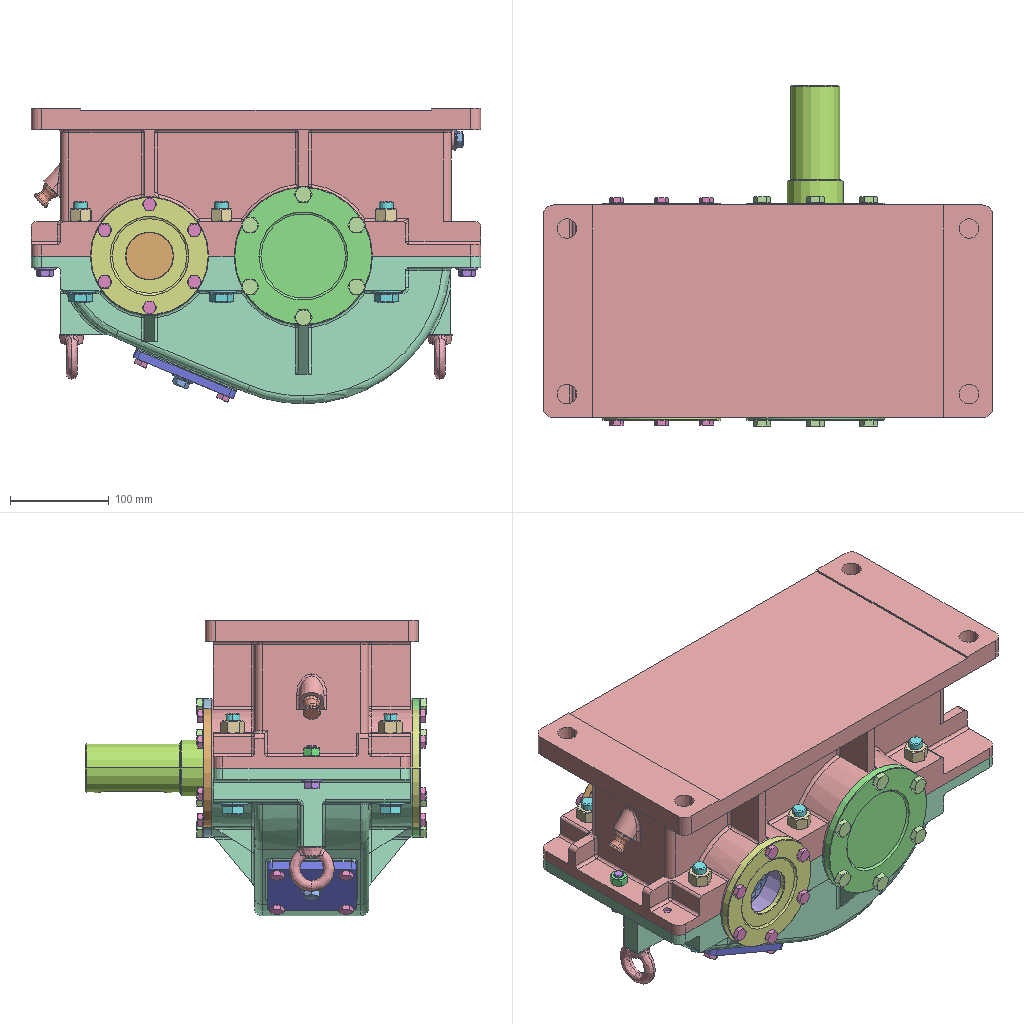Assembly | SolidWorks | 26 different items | 28 placed | box 456 x 346 x 300 mm
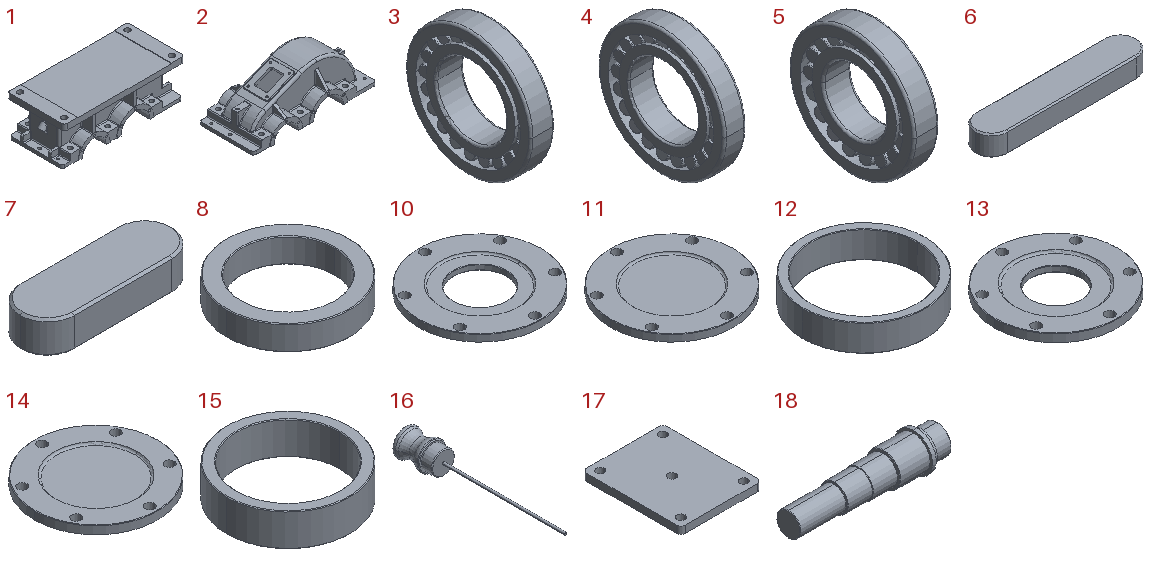Parts list (item | name | quantity | size | volume | features):
1 | - | x1 | 456 x 216 x 150 mm | 3465010 mm3 | features Fillet 25, ICE 15, 3DProfileFeature 4, HoleWzd 4, Chamfer 1, Extrusion 1, MirrorPattern 1, Sweep 1
2 | - | x1 | 456 x 204 x 150 mm | 1972353 mm3 | features Fillet 21, ICE 16, 3DProfileFeature 4, HoleWzd 4, Extrusion 1, MirrorPattern 1
3 | - | x1 | 21.75 x 90 x 90 mm | 63957 mm3 | features Revolution 3, CirPattern 1
4 | - | x1 | 23.75 x 110 x 110 mm | 105381 mm3 | features Revolution 3, CirPattern 1
5 | - | x1 | 19.75 x 80 x 80 mm | 50008 mm3 | features Revolution 3, CirPattern 1
6 | - | x1 | 70 x 14 x 9 mm | 8386 mm3 | features Boss 2, Chamfer 1, Extrusion 1
7 | - | x1 | 56 x 20 x 12 mm | 12325 mm3 | features Boss 2, Chamfer 1, Extrusion 1
8 | - | x1 | 80 x 80 x 16 mm | 35076 mm3 | features Chamfer 1, Extrusion 1
9 | - | x1 | - | - | features ICE 4, Boss 3, CirPattern 3, Cut 2, Fillet 2, Helix 2, SweepCut 2, Chamfer 1, Revolution 1
10 | - | x1 | 140 x 140 x 13 mm | 97648 mm3 | features ICE 3, Chamfer 2, Extrusion 1, Fillet 1
11 | - | x1 | 140 x 140 x 13 mm | 114660 mm3 | features ICE 2, Chamfer 1, Extrusion 1, Fillet 1
12 | - | x2 | 110 x 110 x 24 mm | 57801 mm3 | features Chamfer 1, Extrusion 1
13 | - | x1 | 120 x 120 x 13 mm | 73283 mm3 | features ICE 3, Chamfer 2, Extrusion 1, Fillet 1
14 | - | x1 | 120 x 120 x 13 mm | 84178 mm3 | features ICE 2, Chamfer 1, Extrusion 1, Fillet 1
15 | - | x2 | 90 x 90 x 24 mm | 46523 mm3 | features Chamfer 1, Extrusion 1
16 | - | x1 | 18 x 105 x 18 mm | 4726 mm3 | features Chamfer 2, Fillet 1, Revolution 1
17 | - | x1 | 90 x 110 x 8 mm | 76484 mm3 | features 3DProfileFeature 1, Extrusion 1, HoleWzd 1
18 | - | x1 | 312 x 80 x 80 mm | 861601 mm3 | features Chamfer 4, Fillet 2, ICE 2, Revolution 1
19 | eyebolts gb | x1 | - | - | -
20 | hex flange bolts-heavy grade b gb | x1 | - | - | -
21 | hex nuts, style 1-grades ab gb | x1 | - | - | -
22 | hexagon head bolts-full thread gb | x1 | - | - | -
23 | parallel pins hardening steel gb | x1 | - | - | -
24 | plain parallel keys | x1 | - | - | -
25 | tapered roller bearings gb | x1 | - | - | -
26 | QB.step | x1 | - | - | -
Mates (type | each side: item.copy, entity, surface, feature):
Concentric | 1.1 face cylinder Cut-Extrude1 | 18.1 face cylinder Revolve3
Parallel | 1.1 face plane Boss-Extrude1 | 18.1 face plane Cut-Extrude1
Concentric | 18.1 face cylinder Revolve3 | 8.1 face cylinder Boss-Extrude1
Concentric | 1.1 face cylinder Mirror1 | 14.1 face cylinder Boss-Extrude1
Concentric | 1.1 face cylinder Cut-Extrude1 | 14.1 face cylinder Boss-Extrude1
Coincident | 1.1 face plane Boss-Extrude5 | 14.1 face plane Boss-Extrude1
Concentric | 1.1 face cylinder M10 Tapped Hole1 | 11.1 face cylinder Boss-Extrude1
Concentric | 1.1 face cylinder Cut-Extrude1 | 11.1 face cylinder Boss-Extrude1
Coincident | 1.1 face plane Boss-Extrude5 | 11.1 face plane Boss-Extrude1
Concentric | 1.1 face cylinder Mirror1 | 10.1 face cylinder Boss-Extrude1
Concentric | 18.1 face cylinder Revolve3 | 10.1 face cylinder Boss-Extrude1
Coincident | 1.1 face plane Boss-Extrude5 | 10.1 face plane Boss-Extrude1
Concentric | 1.1 face cylinder M8 Tapped Hole1 | 13.1 face cylinder Boss-Extrude1
Concentric | 15.1 face cylinder Boss-Extrude1 | 13.1 face cylinder Boss-Extrude1
Coincident | 1.1 face plane Boss-Extrude5 | 13.1 face plane Boss-Extrude1
Coincident | 1.1 face plane Boss-Extrude1 | 2.1 face plane Boss-Extrude1
Concentric | 1.1 face cylinder Cut-Extrude4 | 2.1 face cylinder Cut-Extrude4 | 2 times
Concentric | 1.1 face cylinder Size mm Hidden Pin Hole1 | 16.1 face cylinder Revolve1
Coincident | 1.1 face plane Sweep1 | 16.1 face plane Revolve1
Coincident | 2.1 face plane Boss-Extrude11 | 17.1 face plane Boss-Extrude1
Concentric | 2.1 face cylinder M8 Tapped Hole1 | 17.1 face cylinder Boss-Extrude1
Parallel | 2.1 face cylinder M8 Tapped Hole1 | 17.1 face cylinder Boss-Extrude1 | 2 times
Parallel | 2.1 face plane Boss-Extrude11 | 17.1 face plane Boss-Extrude1